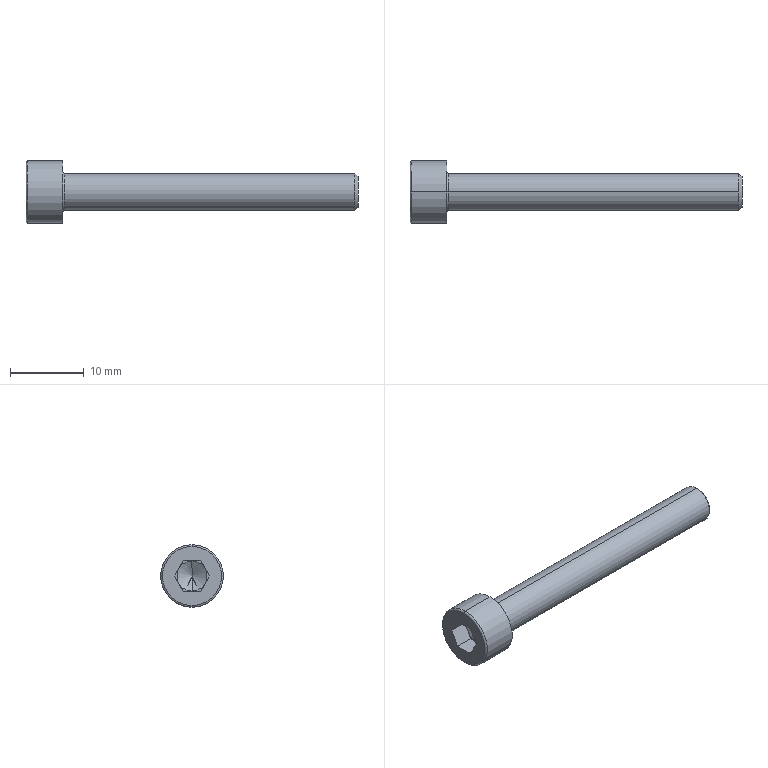Part | STEP file | socket head cap screw_iso_ISO 4762 M5 x 40 --- 22N | 1 solid | 27 faces | box 45 x 8.5 x 8.5 mm | volume 1026 mm3 | plane 15 | cone 4 | torus 4 | cylinder 4 | commonest cylinder face diameters 5 x2 8.5 x2